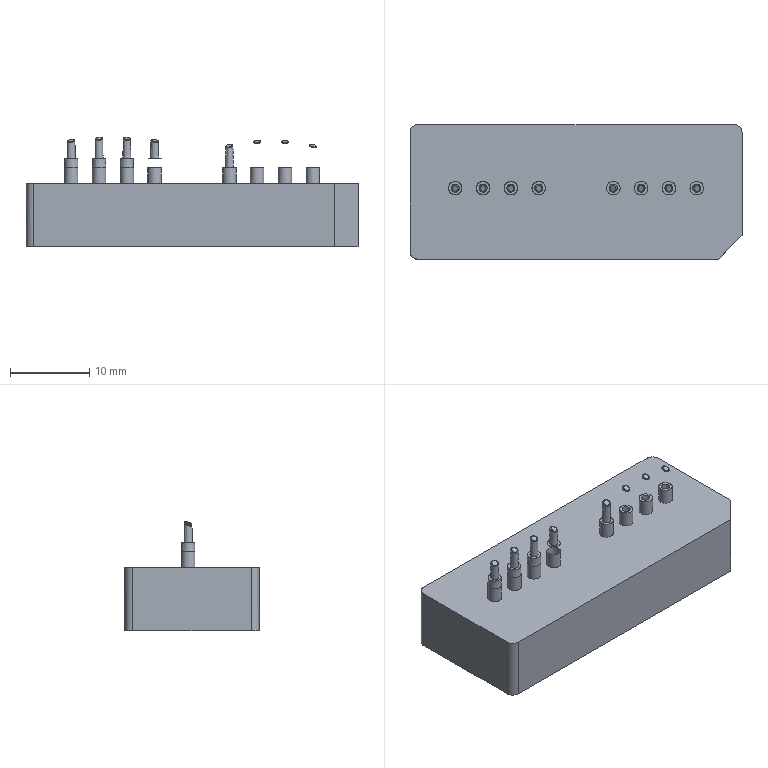NC program | PowerMill | posted by the shop | part box 42 x 17 x 13.856 mm
Lines 12635 to 14179 of 273708:
( TOOL ID   D1.5C_1_1 )
( TOOL DIA. 1.5 TIP RAD 0 LENGTH 61.02 )
( Z = -5.95 )
T26 M6
T3
G91 G28 Z0
G0 G90 G54
M08
S20000 M3
X0 Y0 M8
G43 Z9.805 H26
X5.72 Y1.423
Z.021
G1 Z-1.179 F1800
X5.708 Y1.415 F3000
G3 X5.677 Y1.224 I.08 J-.11
G1 X5.791 Y1.067
X5.904 Y.742
X5.915 Y.445
X5.827 Y.148
X5.757 Y.054
X7.176 Y-.389
X7.188 Y-.381
G3 X7.223 Y-.191 I-.077 J.112
G1 X7.219 Y-.185
X7.188 Y-.148
X7.062 Y.148
X7.015 Y.445
X7.047 Y.742
X7.15 Y1.039
X7.22 Y1.135
X7.276 Y1.224
X7.301 Y1.247
X7.315 Y1.265
X5.678 Y1.482 Z-1.228
X5.666 Y1.473
G3 X5.638 Y1.283 I.081 J-.109
G1 X5.791 Y1.078
X5.921 Y.742
X5.94 Y.445
X5.877 Y.148
X5.791 Y-.021
X5.733 Y-.096
X7.214 Y-.458
X7.227 Y-.449
G3 X7.263 Y-.26 I-.076 J.113
G1 X7.187 Y-.148
X7.061 Y.148
X7.014 Y.445
X7.047 Y.742
X7.149 Y1.039
X7.227 Y1.146
X7.276 Y1.224
X7.298 Y1.244
X7.316 Y1.268
X5.679 Y1.483 Z-1.277
X5.667 Y1.474
G3 X5.64 Y1.283 I.082 J-.109
G1 X5.791 Y1.081
X5.922 Y.742
X5.947 Y.445
X5.898 Y.148
X5.791 Y-.089
X5.682 Y-.2
X7.279 Y-.503
X7.29 Y-.493
G3 X7.294 Y-.3 I-.094 J.099
G1 X7.276 Y-.281
X7.186 Y-.148
X7.06 Y.148
X7.013 Y.445
X7.046 Y.742
X7.148 Y1.039
X7.234 Y1.157
X7.276 Y1.224
X7.295 Y1.241
X7.316 Y1.269
G0 Z2.873
G1 X7.301 Y-.528 F10000
G0 Z-.127
G1 Z-1.327 F1800
X7.312 Y-.517 F3000
G3 X7.317 Y-.325 I-.094 J.099
G1 X7.276 Y-.282
X7.185 Y-.148
X7.059 Y.148
X7.012 Y.445
X7.046 Y.742
X7.147 Y1.039
X7.241 Y1.168
X7.276 Y1.223
X7.292 Y1.238
X7.315 Y1.27
X5.68 Y1.484
X5.668 Y1.475
G3 X5.641 Y1.284 I.082 J-.109
G1 X5.791 Y1.083
X5.922 Y.742
X5.948 Y.445
X5.908 Y.148
X5.791 Y-.118
X5.652 Y-.265
X7.306 Y-.533 Z-1.376
X7.317 Y-.523
G3 X7.322 Y-.33 I-.094 J.099
G1 X7.276 Y-.282
X7.19 Y-.156
X7.184 Y-.148
X7.059 Y.148
X7.011 Y.445
X7.045 Y.742
X7.146 Y1.039
X7.248 Y1.179
X7.276 Y1.223
X7.289 Y1.235
X7.315 Y1.271
X5.682 Y1.485
X5.669 Y1.476
G3 X5.642 Y1.285 I.082 J-.109
G1 X5.791 Y1.086
X5.923 Y.742
X5.949 Y.445
X5.908 Y.148
X5.783 Y-.148
X5.63 Y-.319
X7.307 Y-.534 Z-1.425
X7.318 Y-.524
G3 X7.323 Y-.331 I-.094 J.099
G1 X7.276 Y-.282
X7.195 Y-.163
X7.183 Y-.148
X7.058 Y.148
X7.01 Y.445
X7.045 Y.742
X7.145 Y1.039
X7.256 Y1.191
X7.277 Y1.223
X7.286 Y1.232
X7.315 Y1.272
X5.683 Y1.486
X5.671 Y1.476
G3 X5.643 Y1.286 I.082 J-.109
G1 X5.791 Y1.088
X5.924 Y.742
X5.95 Y.445
X5.908 Y.148
X5.791 Y-.135
X5.787 Y-.142
X5.783 Y-.148
X5.755 Y-.18
X5.634 Y-.328
X7.308 Y-.535 Z-1.474
X7.319 Y-.525
G3 X7.324 Y-.332 I-.094 J.099
G1 X7.276 Y-.282
X7.2 Y-.17
X7.182 Y-.148
X7.058 Y.148
X7.01 Y.445
X7.045 Y.742
X7.144 Y1.039
X7.263 Y1.202
X7.277 Y1.223
X7.283 Y1.229
X7.314 Y1.272
X5.685 Y1.485
X5.673 Y1.476
G3 X5.645 Y1.286 I.081 J-.109
G1 X5.791 Y1.09
X5.925 Y.742
X5.951 Y.445
X5.909 Y.148
X5.791 Y-.136
X5.787 Y-.142
X5.783 Y-.148
X5.76 Y-.174
X5.633 Y-.33
G0 Z2.677
G1 X5.686 Y1.485 F10000
G0 Z-.323
G1 Z-1.523 F1800
X5.674 Y1.476 F3000
G3 X5.646 Y1.285 I.081 J-.109
G1 X5.791 Y1.091
X5.926 Y.742
X5.952 Y.445
X5.909 Y.148
X5.791 Y-.136
X5.785 Y-.144
X5.783 Y-.148
X5.764 Y-.17
X5.632 Y-.332
X7.309 Y-.536
X7.32 Y-.525
G3 X7.325 Y-.333 I-.094 J.099
G1 X7.276 Y-.282
X7.205 Y-.178
X7.181 Y-.148
X7.057 Y.148
X7.009 Y.445
X7.044 Y.742
X7.143 Y1.039
X7.27 Y1.212
X7.277 Y1.223
X7.28 Y1.227
X7.284 Y1.232
X7.312 Y1.271
X5.688 Y1.484 Z-1.573
X5.676 Y1.475
G3 X5.648 Y1.285 I.081 J-.109
G1 X5.791 Y1.091
X5.927 Y.742
X5.953 Y.445
X5.909 Y.148
X5.893 Y.112
X5.791 Y-.136
X5.788 Y-.139
X5.785 Y-.148
X5.632 Y-.334
X7.306 Y-.536
X7.317 Y-.526
G3 X7.325 Y-.334 I-.092 J.1
G1 X7.249 Y-.244
X7.18 Y-.148
X7.057 Y.148
X7.008 Y.445
X7.043 Y.742
X7.142 Y1.039
X7.276 Y1.223
X7.277
Y1.224
X7.278 Y1.225
X7.311 Y1.271
G0 Z2.578
G1 X7.305 Y-.537 F10000
G0 Z-.422
G1 Z-1.622 F1800
X7.316 Y-.527 F3000
G3 X7.326 Y-.334 I-.091 J.101
G1 X7.249 Y-.244
X7.179 Y-.148
X7.056 Y.148
X7.007 Y.445
X7.043 Y.742
X7.141 Y1.039
X7.31 Y1.27
X5.689 Y1.485
X5.676 Y1.476
G3 X5.648 Y1.286 I.081 J-.109
G1 X5.791 Y1.092
X5.928 Y.742
X5.954 Y.445
X5.909 Y.148
X5.845 Y-.006
X5.791 Y-.136
X5.79 Y-.137
X5.786 Y-.148
X5.631 Y-.336
X7.305 Y-.537 Z-1.671
X7.316 Y-.527
G3 X7.327 Y-.335 I-.091 J.101
G1 X7.25 Y-.244
X7.178 Y-.148
X7.056 Y.148
X7.006 Y.445
X7.042 Y.742
X7.14 Y1.039
X7.309 Y1.27
X5.689 Y1.486
X5.677 Y1.477
G3 X5.648 Y1.287 I.081 J-.109
G1 X5.791 Y1.093
X5.928 Y.742
X5.955 Y.445
X5.909 Y.148
X5.791 Y-.14
X5.788 Y-.144
X5.786 Y-.148
X5.64 Y-.326
X5.63 Y-.337
X7.325 Y-.538 Z-1.72
X7.335 Y-.526
G3 X7.326 Y-.334 I-.101 J.092
G1 X7.271 Y-.275
X7.226 Y-.208
X7.177 Y-.148
X7.055 Y.148
X7.005 Y.445
X7.041 Y.742
X7.139 Y1.039
X7.307 Y1.269
X5.689 Y1.487
X5.677 Y1.478
G3 X5.648 Y1.288 I.081 J-.11
G1 X5.791 Y1.094
X5.929 Y.742
X5.956 Y.445
X5.91 Y.148
X5.791 Y-.141
X5.786 Y-.148
X5.785
X5.78 Y-.155
X5.631 Y-.337
X7.325 Y-.537 Z-1.769
X7.335 Y-.526
G3 X7.326 Y-.333 I-.101 J.091
G1 X7.274 Y-.279
X7.231 Y-.216
X7.176 Y-.148
X7.055 Y.148
X7.004 Y.445
X7.041 Y.742
X7.138 Y1.039
X7.309 Y1.272
X5.69 Y1.487
X5.678 Y1.478
G3 X5.649 Y1.288 I.081 J-.11
G1 X5.791 Y1.095
X5.93 Y.742
X5.956 Y.445
X5.91 Y.148
X5.791 Y-.143
X5.632 Y-.338
X7.326 Y-.537 Z-1.819
X7.336 Y-.526
G3 X7.326 Y-.333 I-.102 J.091
G1 X7.277 Y-.282
X7.237 Y-.224
X7.175 Y-.148
X7.054 Y.148
X7.004 Y.445
X7.04 Y.742
X7.137 Y1.039
X7.313 Y1.279
X5.687 Y1.493
X5.675 Y1.485
G3 X5.646 Y1.294 I.08 J-.11
G1 X5.791 Y1.096
X5.931 Y.742
X5.957 Y.445
X5.911 Y.148
X5.791 Y-.145
X5.632 Y-.339
X7.303 Y-.515 Z-1.868
X7.335 Y-.478
X7.361 Y-.404
X7.326 Y-.334
X7.28 Y-.286
X7.242 Y-.232
X7.174 Y-.148
X7.054 Y.148
X7.003 Y.445
X7.039 Y.742
X7.137 Y1.039
X7.313 Y1.28
X5.688 Y1.495
X5.676 Y1.486
G3 X5.646 Y1.295 I.08 J-.11
G1 X5.791 Y1.097
X5.932 Y.742
X5.958 Y.445
X5.912 Y.148
X5.791 Y-.147
X5.633 Y-.34
X7.325 Y-.538 Z-1.917
X7.335 Y-.527
G3 X7.326 Y-.335 I-.101 J.092
G1 X7.284 Y-.29
X7.248 Y-.24
X7.173 Y-.148
X7.053 Y.148
X7.002 Y.445
X7.039 Y.742
X7.136 Y1.039
X7.313 Y1.281
X5.688 Y1.496
X5.676 Y1.487
G3 X5.646 Y1.297 I.08 J-.11
G1 X5.791 Y1.098
X5.932 Y.742
X5.959 Y.445
X5.913 Y.148
X5.791 Y-.148
X5.633 Y-.341
X7.296 Y-.537 Z-1.966
X7.308 Y-.528
G3 X7.326 Y-.336 I-.087 J.105
G1 X7.311 Y-.318
X7.277 Y-.282
X7.253 Y-.248
X7.172 Y-.148
X7.053 Y.148
X7.001 Y.445
X7.038 Y.742
X7.135 Y1.039
X7.312 Y1.282
X5.689 Y1.497
X5.677 Y1.488
G3 X5.646 Y1.298 I.08 J-.11
G1 X5.791 Y1.099
X5.933 Y.742
X5.96 Y.445
X5.914 Y.148
X5.792 Y-.148
X5.633 Y-.342
X7.296 Y-.538 Z-2.015
X7.307 Y-.529
G3 X7.326 Y-.337 I-.086 J.105
G1 X7.303 Y-.309
X7.277 Y-.282
X7.259 Y-.256
X7.171 Y-.148
X7.053 Y.148
X7. Y.445
X7.038 Y.742
X7.134 Y1.039
X7.311 Y1.282
X5.69 Y1.496
X5.678 Y1.487
G3 X5.648 Y1.297 I.08 J-.11
G1 X5.791 Y1.099
X5.934 Y.742
X5.961 Y.445
X5.915 Y.148
X5.793 Y-.148
X5.634 Y-.343
X7.295 Y-.54 Z-2.065
X7.307 Y-.53
G3 X7.326 Y-.338 I-.086 J.105
G1 X7.294 Y-.3
X7.277 Y-.282
X7.265 Y-.264
X7.17 Y-.148
X7.052 Y.148
X6.999 Y.445
X7.037 Y.742
X7.133 Y1.039
X7.312 Y1.284
X5.69 Y1.499
X5.678 Y1.49
G3 X5.647 Y1.3 I.08 J-.11
G1 X5.791 Y1.1
X5.935 Y.742
X5.961 Y.445
X5.916 Y.148
X5.794 Y-.148
X5.634 Y-.344
X7.295 Y-.541 Z-2.114
X7.307 Y-.531
G3 X7.325 Y-.34 I-.086 J.105
G1 X7.286 Y-.291
X7.277 Y-.282
X7.271 Y-.273
X7.169 Y-.148
X7.052 Y.148
X6.998 Y.445
X7.036 Y.742
X7.132 Y1.039
X7.311 Y1.283
X5.691 Y1.498
X5.679 Y1.49
G3 X5.648 Y1.3 I.08 J-.11
G1 X5.791 Y1.101
X5.936 Y.742
X5.962 Y.445
X5.917 Y.148
X5.795 Y-.148
X5.634 Y-.344
G0 Z2.037
G1 X5.693 Y1.498 F10000
G0 Z-.963
G1 Z-2.163 F1800
X5.681 Y1.489 F3000
G3 X5.65 Y1.299 I.079 J-.111
G1 X5.791 Y1.102
X5.936 Y.742
X5.963 Y.445
X5.918 Y.148
X5.796 Y-.148
X5.634 Y-.345
X7.295 Y-.542
X7.306 Y-.532
G3 X7.325 Y-.341 I-.086 J.105
G1 X7.279 Y-.284
X7.278 Y-.283
X7.277 Y-.282
X7.276 Y-.281
X7.168 Y-.148
X7.051 Y.148
X6.998 Y.445
X7.036 Y.742
X7.131 Y1.039
X7.309 Y1.283
G0 Z2.495
G1 X7.294 Y-.543 F10000
G0 Z-1.012
G1 Z-2.212 F1800
X7.306 Y-.533 F3000
G3 X7.325 Y-.342 I-.086 J.105
G1 X7.167 Y-.148
X7.051 Y.148
X6.997 Y.445
X7.035 Y.742
X7.13 Y1.039
X7.308 Y1.282
X5.694 Y1.498
X5.682 Y1.489
G3 X5.65 Y1.299 I.079 J-.111
G1 X5.791 Y1.103
X5.937 Y.742
X5.964 Y.445
X5.918 Y.148
X5.797 Y-.148
X5.635 Y-.346
X7.294 Y-.544 Z-2.261
X7.306 Y-.534
G3 X7.325 Y-.343 I-.086 J.105
G1 X7.166 Y-.148
X7.05 Y.148
X6.996 Y.445
X7.034 Y.742
X7.129 Y1.039
X7.311 Y1.287
X5.692 Y1.503
X5.68 Y1.494
G3 X5.648 Y1.305 I.079 J-.111
G1 X5.791 Y1.103
X5.938 Y.742
X5.965 Y.445
X5.919 Y.148
X5.849 Y-.02
X5.797 Y-.148
X5.796 Y-.15
X5.791 Y-.161
X5.635 Y-.348
X7.294 Y-.545 Z-2.311
X7.306 Y-.536
G3 X7.325 Y-.344 I-.086 J.105
G1 X7.165 Y-.148
X7.05 Y.148
X6.995 Y.445
X7.034 Y.742
X7.128 Y1.039
X7.31 Y1.287
X5.694 Y1.503
X5.681 Y1.494
G3 X5.649 Y1.304 I.079 J-.111
G1 X5.791 Y1.104
X5.939 Y.742
X5.966 Y.445
X5.92 Y.148
X5.791 Y-.163
X5.636 Y-.349
X7.294 Y-.546 Z-2.36
X7.305 Y-.537
G3 X7.324 Y-.345 I-.086 J.105
G1 X7.164 Y-.148
X7.049 Y.148
X6.994 Y.445
X7.033 Y.742
X7.127 Y1.039
X7.276 Y1.251
X7.299 Y1.273
X7.309 Y1.286
X5.695 Y1.502
X5.683 Y1.494
G3 X5.65 Y1.304 I.079 J-.111
G1 X5.791 Y1.105
X5.94 Y.742
X5.967 Y.445
X5.921 Y.148
X5.791 Y-.164
X5.636 Y-.35
X7.293 Y-.547 Z-2.409
X7.305 Y-.537
G3 X7.324 Y-.346 I-.086 J.105
G1 X7.163 Y-.148
X7.049 Y.148
X6.993 Y.445
X7.033 Y.742
X7.126 Y1.039
X7.276 Y1.252
X7.303 Y1.277
X7.309 Y1.285
X5.696 Y1.503
X5.684 Y1.494
G3 X5.651 Y1.305 I.078 J-.111
G1 X5.791 Y1.106
X5.94 Y.742
X5.967 Y.445
X5.922 Y.148
X5.791 Y-.166
X5.636 Y-.351
G0 Z2.088
G1 X5.696 Y1.504 F10000
G0 Z-1.258
G1 Z-2.458 F1800
X5.684 Y1.496 F3000
G3 X5.651 Y1.306 I.078 J-.111
G1 X5.791 Y1.106
X5.941 Y.742
X5.968 Y.445
X5.923 Y.148
X5.802 Y-.148
X5.795 Y-.157
X5.791 Y-.166
X5.636 Y-.35
X7.292 Y-.548
X7.304 Y-.538
G3 X7.323 Y-.346 I-.086 J.105
G1 X7.162 Y-.148
X7.048 Y.148
X6.992 Y.445
X7.032 Y.742
X7.125 Y1.039
X7.276 Y1.253
X7.306 Y1.281
X7.308 Y1.284
G0 Z2.561
G1 X7.292 Y-.548 F10000
G0 Z-1.307
G1 Z-2.507 F1800
X7.303 Y-.539 F3000
G3 X7.323 Y-.347 I-.086 J.105
G1 X7.161 Y-.148
X7.047 Y.148
X6.992 Y.445
X7.031 Y.742
X7.124 Y1.039
X7.276 Y1.255
X7.307 Y1.284
X5.697 Y1.506
X5.685 Y1.497
G3 X5.651 Y1.307 I.078 J-.112
G1 X5.791 Y1.107
X5.942 Y.742
X5.969 Y.445
X5.924 Y.148
X5.803 Y-.148
X5.794 Y-.159
X5.791 Y-.166
X5.654 Y-.33
X5.636 Y-.351
X7.291 Y-.549 Z-2.556
X7.303 Y-.539
G3 X7.322 Y-.348 I-.086 J.105
G1 X7.16 Y-.148
X7.046 Y.148
X6.991 Y.445
X7.031 Y.742
X7.123 Y1.039
X7.276 Y1.256
X7.307 Y1.285
X5.697 Y1.507
X5.685 Y1.498
G3 X5.651 Y1.309 I.078 J-.112
G1 X5.791 Y1.108
X5.943 Y.742
X5.97 Y.445
X5.925 Y.148
X5.804 Y-.148
X5.793 Y-.162
X5.791 Y-.166
X5.704 Y-.27
X5.636 Y-.352
X7.291 Y-.55 Z-2.606
X7.302 Y-.54
G3 X7.322 Y-.349 I-.086 J.106
G1 X7.159 Y-.148
X7.045 Y.148
X6.99 Y.445
X7.03 Y.742
X7.122 Y1.039
X7.276 Y1.257
X7.307 Y1.286
X5.705 Y1.5
X5.692 Y1.491
G3 X5.657 Y1.302 I.077 J-.112
G1 X5.69 Y1.253
X5.791 Y1.108
X5.794 Y1.1
X5.836 Y1.039
X5.944 Y.742
X5.971 Y.445
X5.926 Y.148
X5.805 Y-.148
X5.796 Y-.159
X5.793 Y-.162
X5.791 Y-.166
X5.756 Y-.208
X5.637 Y-.353
X7.289 Y-.549 Z-2.655
X7.301 Y-.54
G3 X7.32 Y-.348 I-.086 J.106
G1 X7.158 Y-.148
X7.044 Y.148
X6.989 Y.445
X7.029 Y.742
X7.121 Y1.039
X7.276 Y1.258
X7.307 Y1.287
X5.705 Y1.5
X5.693 Y1.492
G3 X5.657 Y1.303 I.077 J-.112
G1 X5.744 Y1.175
X5.791 Y1.108
X5.793 Y1.104
X5.837 Y1.039
X5.944 Y.742
X5.972 Y.445
X5.926 Y.148
X5.806 Y-.148
X5.638 Y-.352
G0 Z2.026
G1 X5.706 Y1.501 F10000
G0 Z-1.504
G1 Z-2.704 F1800
X5.693 Y1.493 F3000
G3 X5.657 Y1.304 I.077 J-.112
G1 X5.838 Y1.039
X5.945 Y.742
X5.972 Y.445
X5.927 Y.148
X5.807 Y-.148
X5.64 Y-.351
X7.287 Y-.548
X7.299 Y-.539
G3 X7.318 Y-.347 I-.086 J.106
G1 X7.157 Y-.148
X7.043 Y.148
X6.988 Y.445
X7.028 Y.742
X7.12 Y1.039
X7.276 Y1.259
X7.307 Y1.288
X5.706 Y1.502 Z-2.753
X5.694 Y1.494
G3 X5.658 Y1.305 I.077 J-.113
G1 X5.839 Y1.039
X5.946 Y.742
X5.973 Y.445
X5.928 Y.148
X5.808 Y-.148
X5.641 Y-.351
X7.285 Y-.548
X7.297 Y-.538
G3 X7.317 Y-.347 I-.086 J.106
G1 X7.156 Y-.148
X7.043 Y.148
X6.987 Y.445
X7.027 Y.742
X7.119 Y1.039
X7.276 Y1.261
X7.306 Y1.289
X5.707 Y1.503 Z-2.802
X5.694 Y1.495
G3 X5.658 Y1.306 I.077 J-.113
G1 X5.84 Y1.039
X5.947 Y.742
X5.974 Y.445
X5.929 Y.148
X5.809 Y-.148
X5.641 Y-.351
X7.284 Y-.547
X7.295 Y-.538
G3 X7.315 Y-.346 I-.086 J.106
G1 X7.155 Y-.148
X7.042 Y.148
X6.986 Y.445
X7.027 Y.742
X7.118 Y1.039
X7.276 Y1.262
X7.306 Y1.29
X5.707 Y1.504 Z-2.851
X5.695 Y1.496
G3 X5.659 Y1.307 I.077 J-.113
G1 X5.841 Y1.039
X5.947 Y.742
X5.975 Y.445
X5.93 Y.148
X5.809 Y-.148
X5.641 Y-.352
X7.282 Y-.547
X7.294 Y-.537
G3 X7.314 Y-.346 I-.086 J.106
G1 X7.154 Y-.148
X7.041 Y.148
X6.986 Y.445
X7.026 Y.742
X7.117 Y1.039
X7.276 Y1.263
X7.306 Y1.291
X5.708 Y1.505 Z-2.899
X5.695 Y1.497
G3 X5.659 Y1.308 I.077 J-.113
G1 X5.842 Y1.039
X5.948 Y.742
X5.976 Y.445
X5.931 Y.148
X5.81 Y-.148
X5.641 Y-.353
X7.285 Y-.552
X7.297 Y-.543
G3 X7.317 Y-.351 I-.086 J.106
G1 X7.153 Y-.148
X7.04 Y.148
X6.985 Y.445
X7.025 Y.742
X7.116 Y1.039
X7.276 Y1.264
X7.306 Y1.292
X5.708 Y1.506 Z-2.947
X5.696 Y1.498
G3 X5.66 Y1.309 I.076 J-.113
G1 X5.843 Y1.039
X5.949 Y.742
X5.977 Y.445
X5.932 Y.148
X5.811 Y-.148
X5.641 Y-.354
X7.279 Y-.546
X7.291 Y-.536
G3 X7.311 Y-.345 I-.086 J.106
G1 X7.152 Y-.148
X7.039 Y.148
X6.984 Y.445
X7.024 Y.742
X7.115 Y1.039
X7.276 Y1.266
X7.305 Y1.293
X5.709 Y1.507 Z-2.995
X5.696 Y1.499
G3 X5.66 Y1.31 I.076 J-.113
G1 X5.843 Y1.039
X5.95 Y.742
X5.977 Y.445
X5.933 Y.148
X5.812 Y-.148
X5.641 Y-.355
X7.279 Y-.547
X7.291 Y-.537
G3 X7.311 Y-.346 I-.086 J.106
G1 X7.151 Y-.148
X7.038 Y.148
X6.983 Y.445
X7.023 Y.742
X7.115 Y1.039
X7.276 Y1.267
X7.305 Y1.294
X5.709 Y1.508 Z-3.044
X5.697 Y1.5
G3 X5.661 Y1.311 I.076 J-.113
G1 X5.844 Y1.039
X5.951 Y.742
X5.978 Y.445
X5.934 Y.148
X5.813 Y-.148
X5.641 Y-.356
X7.278 Y-.548
X7.29 Y-.538
G3 X7.31 Y-.347 I-.086 J.106
G1 X7.15 Y-.148
X7.038 Y.148
X6.982 Y.445
X7.022 Y.742
X7.114 Y1.039
X7.276 Y1.268
X7.305 Y1.295
X5.71 Y1.509 Z-3.092
X5.697 Y1.501
G3 X5.661 Y1.312 I.076 J-.113
G1 X5.845 Y1.039
X5.951 Y.742
X5.979 Y.445
X5.934 Y.148
X5.814 Y-.148
X5.642 Y-.357
X7.278 Y-.549
X7.29 Y-.54
G3 X7.31 Y-.348 I-.086 J.106
G1 X7.149 Y-.148
X7.037 Y.148
X6.981 Y.445
X7.022 Y.742
X7.113 Y1.039
X7.276 Y1.269
X7.305 Y1.296
G0 Z2.528
G1 X7.278 Y-.55 F10000
G0 Z-1.94
G1 Z-3.14 F1800
X7.29 Y-.541 F3000
G3 X7.31 Y-.349 I-.086 J.106
G1 X7.148 Y-.148
X7.036 Y.148
X6.981 Y.445
X7.021 Y.742
X7.112 Y1.039
X7.276 Y1.27
X7.304 Y1.297
X5.71 Y1.51
X5.698 Y1.501
G3 X5.661 Y1.312 I.076 J-.113
G1 X5.846 Y1.039
X5.952 Y.742
X5.98 Y.445
X5.935 Y.148
X5.815 Y-.148
X5.642 Y-.358
X7.278 Y-.551 Z-3.188
X7.289 Y-.542
G3 X7.31 Y-.35 I-.086 J.106
G1 X7.147 Y-.148
X7.035 Y.148
X6.98 Y.445
X7.02 Y.742
X7.111 Y1.039
X7.276 Y1.272
X7.304 Y1.298
X5.711 Y1.511
X5.698 Y1.502
G3 X5.662 Y1.313 I.076 J-.113
G1 X5.847 Y1.039
X5.953 Y.742
X5.981 Y.445
X5.936 Y.148
X5.816 Y-.148
X5.642 Y-.359
G0 Z2.074
G1 X5.711 Y1.512 F10000
G0 Z-2.037
G1 Z-3.237 F1800
X5.699 Y1.503 F3000
G3 X5.662 Y1.314 I.076 J-.113
G1 X5.848 Y1.039
X5.954 Y.742
X5.982 Y.445
X5.937 Y.148
X5.817 Y-.148
X5.642 Y-.36
X7.277 Y-.552
X7.289 Y-.543
G3 X7.309 Y-.351 I-.086 J.106
G1 X7.146 Y-.148
X7.034 Y.148
X7.031 Y.171
X6.98 Y.445
X6.985 Y.486
X6.979 Y.526
X7.006 Y.633
X7.02 Y.742
X7.105 Y1.02
X7.11 Y1.039
X7.276 Y1.273
X7.305 Y1.3
X5.712 Y1.513 Z-3.285
X5.699 Y1.504
G3 X5.663 Y1.315 I.076 J-.113
G1 X5.849 Y1.039
X5.954 Y.742
X5.982 Y.445
X5.938 Y.148
X5.818 Y-.148
X5.642 Y-.361
X7.277 Y-.553
X7.289 Y-.544
G3 X7.309 Y-.352 I-.085 J.106
G1 X7.145 Y-.148
X7.033 Y.148
X6.979 Y.43
Y.539
X7.006 Y.64
X7.02 Y.742
X7.098 Y.997
X7.109 Y1.039
X7.276 Y1.274
X7.305 Y1.301
X5.712 Y1.514 Z-3.333
X5.7 Y1.505
G3 X5.663 Y1.316 I.076 J-.113
G1 X5.85 Y1.039
X5.955 Y.742
X5.983 Y.445
X5.939 Y.148
X5.819 Y-.148
X5.642 Y-.361
X7.277 Y-.554
X7.288 Y-.545
G3 X7.309 Y-.353 I-.085 J.106
G1 X7.144 Y-.148
X7.032 Y.148
X6.979 Y.419
Y.55
X7.038 Y.796
X7.108 Y1.039
X7.276 Y1.275
X7.306 Y1.303
X5.713 Y1.515 Z-3.381
X5.7 Y1.506
G3 X5.664 Y1.317 I.076 J-.113
G1 X5.851 Y1.039
X5.956 Y.742
X5.984 Y.445
X5.94 Y.148
X5.82 Y-.148
X5.642 Y-.362
X7.276 Y-.555
X7.288 Y-.546
G3 X7.309 Y-.354 I-.085 J.106
G1 X7.143 Y-.148
X7.032 Y.148
X6.979 Y.41
Y.559
X7.039 Y.8
X7.107 Y1.039
X7.276 Y1.277
X7.307 Y1.305
X5.714 Y1.516 Z-3.43
X5.701 Y1.507
G3 X5.664 Y1.318 I.076 J-.113
G1 X5.852 Y1.039
X5.957 Y.742
X5.985 Y.445
X5.941 Y.148
X5.821 Y-.148
X5.642 Y-.363
X7.276 Y-.556
X7.288 Y-.547
G3 X7.308 Y-.356 I-.085 J.106
G1 X7.142 Y-.148
X7.031 Y.148
X6.979 Y.402
Y.567
X7.014 Y.696
X7.02 Y.742
X7.071 Y.908
X7.106 Y1.039
X7.276 Y1.278
X7.307 Y1.307
X5.714 Y1.517 Z-3.478
X5.702 Y1.508
G3 X5.665 Y1.319 I.076 J-.113
G1 X5.853 Y1.039
X5.957 Y.742
X5.986 Y.445
X5.941 Y.148
X5.821 Y-.148
X5.642 Y-.364
X7.276 Y-.558
X7.287 Y-.548
G3 X7.308 Y-.357 I-.085 J.106
G1 X7.141 Y-.148
X7.03 Y.148
X6.979 Y.394
Y.575
X7.016 Y.71
X7.02 Y.742
X7.059 Y.87
X7.105 Y1.039
X7.276 Y1.279
X7.308 Y1.308
X5.714 Y1.519 Z-3.526
X5.701 Y1.51
G3 X5.664 Y1.322 I.076 J-.113
G1 X5.854 Y1.039
X5.958 Y.742
X5.987 Y.445
X5.942 Y.148
X5.822 Y-.148
X5.642 Y-.365
X7.275 Y-.559
X7.287 Y-.549
G3 X7.308 Y-.358 I-.085 J.106
G1 X7.14 Y-.148
X7.029 Y.148
X6.979 Y.387
Y.582
X7.017 Y.722
X7.02 Y.742
X7.047 Y.828
X7.104 Y1.039
X7.276 Y1.28
X7.31 Y1.312
X5.714 Y1.52 Z-3.574
X5.702 Y1.511
G3 X5.665 Y1.322 I.076 J-.113
G1 X5.855 Y1.039
X5.959 Y.742
X5.987 Y.445
X5.943 Y.148
X5.823 Y-.148
X5.642 Y-.366
X7.275 Y-.56
X7.287 Y-.55
G3 X7.308 Y-.359 I-.085 J.106
G1 X7.139 Y-.148
X7.028 Y.148
X6.979 Y.381
Y.588
X7.019 Y.733
X7.02 Y.742
X7.034 Y.786
X7.103 Y1.039
X7.276 Y1.281
X7.309 Y1.312
X5.715 Y1.521 Z-3.623
X5.702 Y1.512
G3 X5.665 Y1.323 I.076 J-.113
G1 X5.856 Y1.039
X5.96 Y.742
X5.988 Y.445
X5.944 Y.148
X5.824 Y-.148
X5.642 Y-.367
X7.275 Y-.561
X7.286 Y-.551
G3 X7.307 Y-.36 I-.085 J.106
G1 X7.138 Y-.148
X7.027 Y.148
X6.979 Y.375
Y.594
X7.102 Y1.039
X7.276 Y1.283
X7.309 Y1.313
X5.716 Y1.52 Z-3.671
X5.704 Y1.512
G3 X5.667 Y1.323 I.076 J-.113
G1 X5.857 Y1.039
X5.96 Y.742
X5.989 Y.445
X5.945 Y.148
X5.825 Y-.148
X5.642 Y-.368
X7.274 Y-.562
X7.286 Y-.552
G3 X7.307 Y-.361 I-.085 J.106
G1 X7.137 Y-.148
X7.027 Y.148
X6.979 Y.369
Y.6
X7.102 Y1.039
X7.276 Y1.284
X7.307 Y1.312
X5.718 Y1.519 Z-3.719
X5.705 Y1.511
G3 X5.668 Y1.322 I.076 J-.113
G1 X5.858 Y1.039
X5.961 Y.742
X5.99 Y.445
X5.946 Y.148
X5.826 Y-.148
X5.643 Y-.369
X7.274 Y-.563
X7.286 Y-.553
G3 X7.307 Y-.362 I-.085 J.106
G1 X7.136 Y-.148
X7.026 Y.148
X6.979 Y.363
Y.605
X7.101 Y1.039
X7.276 Y1.285
X7.305 Y1.311
X5.719 Y1.519 Z-3.767
X5.707 Y1.51
G3 X5.67 Y1.322 I.076 J-.113
G1 X5.859 Y1.039
X5.962 Y.742
X5.991 Y.445
X5.947 Y.148
X5.827 Y-.148
X5.643 Y-.37
X7.274 Y-.564
X7.285 Y-.554
G3 X7.307 Y-.363 I-.085 J.106
G1 X7.135 Y-.148
X7.025 Y.148
X6.979 Y.356
Y.61
X7.1 Y1.039
X7.276 Y1.286
X7.303 Y1.311
X5.721 Y1.518 Z-3.816
X5.708 Y1.51
G3 X5.671 Y1.321 I.076 J-.113
G1 X5.86 Y1.039
X5.963 Y.742
X5.992 Y.445
X5.947 Y.148
X5.828 Y-.148
X5.643 Y-.371
X7.273 Y-.565
X7.285 Y-.555
G3 X7.306 Y-.364 I-.085 J.106
G1 X7.134 Y-.148
X7.024 Y.148
X6.979 Y.352
Y.615
X7.099 Y1.039
X7.276 Y1.287
X7.301 Y1.31
G0 Z2.479
G1 X7.273 Y-.566 F10000
G0 Z-2.664
G1 Z-3.864 F1800
X7.285 Y-.556 F3000
G3 X7.306 Y-.365 I-.085 J.106
G1 X7.133 Y-.148
X7.023 Y.148
X6.979 Y.347
Y.619
X7.098 Y1.039
X7.276 Y1.289
X7.302 Y1.313
X5.723 Y1.518
X5.71 Y1.509
G3 X5.673 Y1.32 I.076 J-.113
G1 X5.861 Y1.039
X5.964 Y.742
X5.992 Y.445
X5.948 Y.148
X5.875 Y-.037
X5.791 Y-.217
X5.653 Y-.359
X5.642 Y-.373
X7.273 Y-.567 Z-3.912
X7.284 Y-.558
G3 X7.306 Y-.366 I-.085 J.106
G1 X7.132 Y-.148
X7.022 Y.148
X6.979 Y.343
Y.624
X7.097 Y1.039
X7.276 Y1.29
X7.3 Y1.312
X5.724 Y1.517
X5.712 Y1.509
G3 X5.674 Y1.32 I.076 J-.113
G1 X5.862 Y1.039
X5.964 Y.742
X5.993 Y.445
X5.949 Y.148
X5.874 Y-.037
X5.791 Y-.219
X5.644 Y-.369
X5.64 Y-.374
X7.272 Y-.568 Z-3.96
X7.284 Y-.558
G3 X7.305 Y-.367 I-.085 J.106
G1 X7.131 Y-.148
X7.022 Y.148
X6.979 Y.339
Y.629
X7.096 Y1.039
X7.276 Y1.291
X7.3 Y1.313
X5.726 Y1.516
X5.713 Y1.508
G3 X5.676 Y1.319 I.076 J-.113
G1 X5.863 Y1.039
X5.965 Y.742
X5.994 Y.445
X5.95 Y.148
X5.908 Y.051
X5.828 Y-.148
X5.816 Y-.162
X5.791 Y-.221
X5.639 Y-.376
X7.272 Y-.569 Z-4.008
X7.284 Y-.56
G3 X7.305 Y-.368 I-.085 J.106
G1 X7.13 Y-.148
X7.021 Y.148
X6.979 Y.335
Y.634
X7.095 Y1.039
X7.276 Y1.292
X7.299 Y1.313
X5.727 Y1.516
X5.715 Y1.507
G3 X5.677 Y1.319 I.076 J-.113
G1 X5.864 Y1.039
X5.966 Y.742
X5.995 Y.445
X5.951 Y.148
X5.896 Y.02
X5.828 Y-.148
X5.818 Y-.16
X5.791 Y-.222
X5.639 Y-.377
X6.756 Y-.467 Z-4.058
X6.769 Y-.459
G3 X6.817 Y-.273 I-.069 J.117
G1 X6.743 Y-.148
X6.682 Y.018
X6.616 Y.445
X6.638 Y.742
X6.682 Y.929
X6.804 Y1.207
X6.237 Y1.4
X6.224 Y1.393
G3 X6.163 Y1.211 I.061 J-.122
G1 X6.249 Y1.039
X6.323 Y.742
X6.349 Y.445
X6.313 Y.148
X6.223 Y-.148
X6.154 Y-.274
X6.775 Y-.5 Z-4.108
X6.788 Y-.492
G3 X6.836 Y-.306 I-.069 J.117
G1 X6.743 Y-.148
X6.682 Y.017
X6.616 Y.445
X6.638 Y.742
X6.682 Y.929
X6.82 Y1.243
X6.219 Y1.435
X6.206 Y1.429
G3 X6.145 Y1.246 I.061 J-.122
G1 X6.249 Y1.039
X6.323 Y.742
X6.349 Y.445
X6.313 Y.148
X6.223 Y-.148
X6.136 Y-.307
X7.196 Y-.963 Z-4.158
X7.207 Y-.952
G3 X7.202 Y-.76 I-.098 J.094
G1 X6.979 Y-.547
X6.743 Y-.148
X6.682 Y.017
X6.616 Y.445
X6.638 Y.742
X6.682 Y.929
X6.861 Y1.336
X6.979 Y1.502
X7.19 Y1.704
X5.749 Y1.913
X5.741 Y1.901
G3 X5.778 Y1.712 I.113 J-.076
G1 X5.791 Y1.703
X6.1 Y1.336
X6.249 Y1.039
X6.323 Y.742
X6.349 Y.445
X6.313 Y.148
X6.223 Y-.148
X6.06 Y-.445
X5.791 Y-.741
X5.768 Y-.758
X7.196 Y-.963 Z-4.208
X7.207 Y-.952
G3 X7.202 Y-.76 I-.098 J.094
G1 X6.979 Y-.547
X6.743 Y-.148
X6.682 Y.017
X6.616 Y.445
X6.638 Y.742
X6.682 Y.929
X6.861 Y1.336
X6.979 Y1.502
X7.19 Y1.704
X5.749 Y1.913
X5.741 Y1.901
G3 X5.778 Y1.712 I.113 J-.076
G1 X5.791 Y1.703
X6.1 Y1.336
X6.249 Y1.039
X6.323 Y.742
X6.349 Y.445
X6.313 Y.148
X6.223 Y-.148
X6.06 Y-.445
X5.791 Y-.741
X5.768 Y-.758
X7.196 Y-.963 Z-4.257
X7.207 Y-.952
G3 X7.202 Y-.76 I-.098 J.094
G1 X6.979 Y-.547
X6.743 Y-.148
X6.682 Y.017
X6.616 Y.445
X6.638 Y.742
X6.682 Y.929
X6.861 Y1.336
X6.979 Y1.502
X7.19 Y1.704
X5.749 Y1.913
X5.741 Y1.901
G3 X5.778 Y1.712 I.113 J-.076
G1 X5.791 Y1.703
X6.1 Y1.336
X6.249 Y1.039
X6.323 Y.742
X6.349 Y.445
X6.313 Y.148
X6.223 Y-.148
X6.06 Y-.445
X5.791 Y-.741
X5.768 Y-.758
X7.196 Y-.963 Z-4.307
X7.207 Y-.952
G3 X7.202 Y-.76 I-.098 J.094
G1 X6.979 Y-.547
X6.743 Y-.148
X6.682 Y.017
X6.616 Y.445
X6.638 Y.742
X6.682 Y.929
X6.861 Y1.336
X6.979 Y1.502
X7.19 Y1.704
X5.749 Y1.913
X5.741 Y1.901
G3 X5.778 Y1.712 I.113 J-.076
G1 X5.791 Y1.703
X6.1 Y1.336
X6.249 Y1.039
X6.323 Y.742
X6.349 Y.445
X6.313 Y.148
X6.223 Y-.148
X6.06 Y-.445
X5.791 Y-.741
X5.768 Y-.758
X7.196 Y-.963 Z-4.357
X7.207 Y-.952
G3 X7.202 Y-.76 I-.098 J.094
G1 X6.979 Y-.547
X6.743 Y-.148
X6.682 Y.017
X6.616 Y.445
X6.638 Y.742
X6.682 Y.929
X6.861 Y1.336
X6.979 Y1.502
X7.19 Y1.704
X5.749 Y1.913
X5.741 Y1.901
G3 X5.778 Y1.712 I.113 J-.076
G1 X5.791 Y1.703
X6.1 Y1.336
X6.249 Y1.039
X6.323 Y.742
X6.349 Y.445
X6.313 Y.148
X6.223 Y-.148
X6.06 Y-.445
X5.791 Y-.741
X5.768 Y-.758
X7.196 Y-.963 Z-4.407
X7.207 Y-.952
G3 X7.202 Y-.76 I-.098 J.094
G1 X6.979 Y-.547
X6.743 Y-.148
X6.682 Y.017
X6.616 Y.445
X6.638 Y.742
X6.682 Y.929
X6.861 Y1.336
X6.979 Y1.502
X7.19 Y1.704
X5.749 Y1.913
X5.741 Y1.901
G3 X5.778 Y1.712 I.113 J-.076
G1 X5.791 Y1.703
X6.1 Y1.336
X6.249 Y1.039
X6.323 Y.742
X6.349 Y.445
X6.313 Y.148
X6.223 Y-.148
X6.06 Y-.445
X5.791 Y-.741
X5.768 Y-.758
X7.196 Y-.963 Z-4.457
X7.207 Y-.952
G3 X7.202 Y-.76 I-.098 J.094
G1 X6.979 Y-.547
X6.743 Y-.148
X6.682 Y.017
X6.616 Y.445
X6.638 Y.742
X6.682 Y.929
X6.861 Y1.336
X6.979 Y1.502
X7.19 Y1.704
X5.749 Y1.913
X5.741 Y1.901
G3 X5.778 Y1.712 I.113 J-.076
G1 X5.791 Y1.703
X6.1 Y1.336
X6.249 Y1.039
X6.323 Y.742
X6.349 Y.445
X6.313 Y.148
X6.223 Y-.148
X6.06 Y-.445
X5.791 Y-.741
X5.768 Y-.758
X7.196 Y-.963 Z-4.506
X7.207 Y-.952
G3 X7.202 Y-.76 I-.098 J.094
G1 X6.979 Y-.547
X6.743 Y-.148
X6.682 Y.017
X6.616 Y.445
X6.638 Y.742
X6.682 Y.929
X6.861 Y1.336
X6.979 Y1.502
X7.19 Y1.704
X5.749 Y1.913
X5.741 Y1.901
G3 X5.778 Y1.712 I.113 J-.076
G1 X5.791 Y1.703
X6.1 Y1.336
X6.249 Y1.039
X6.323 Y.742
X6.349 Y.445
X6.313 Y.148
X6.223 Y-.148
X6.06 Y-.445
X5.791 Y-.741
X5.768 Y-.758
X7.196 Y-.963 Z-4.556
X7.207 Y-.952
G3 X7.202 Y-.76 I-.098 J.094
G1 X6.979 Y-.547
X6.743 Y-.148
X6.682 Y.017
X6.616 Y.445
X6.638 Y.742
X6.682 Y.929
X6.861 Y1.336
X6.979 Y1.502
X7.19 Y1.704
X5.749 Y1.913
X5.741 Y1.901
G3 X5.778 Y1.712 I.113 J-.076
G1 X5.791 Y1.703
X6.1 Y1.336
X6.249 Y1.039
X6.323 Y.742
X6.349 Y.445